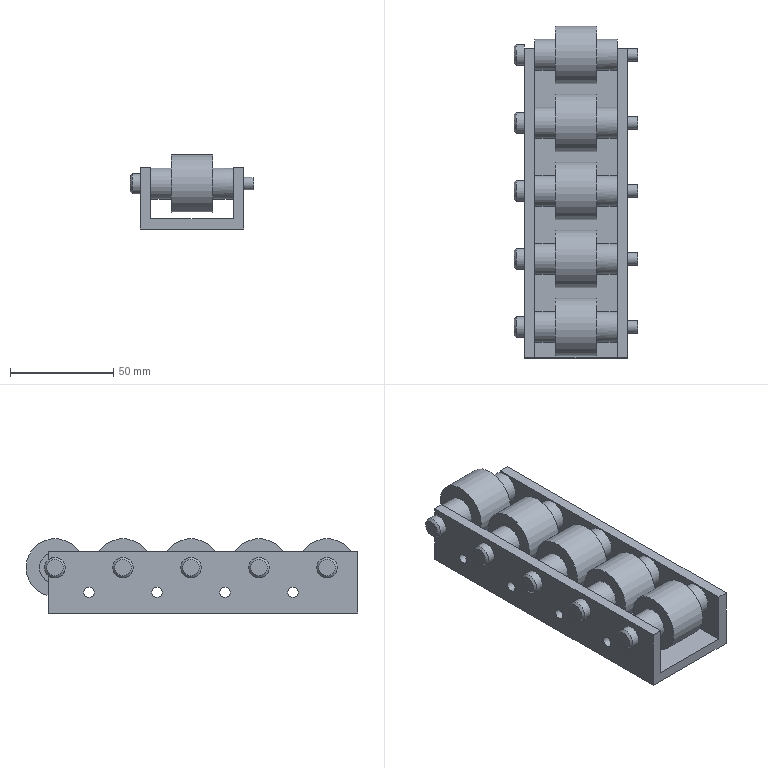Part | NX | features solid 2 | 1 solid | 71 faces | box 60 x 161 x 36 mm | volume 156058 mm3 | plane 33 | cylinder 33 | cone 5 | commonest cylinder face diameters 15 x10 5 x8 6 x5 10 x5 28 x5